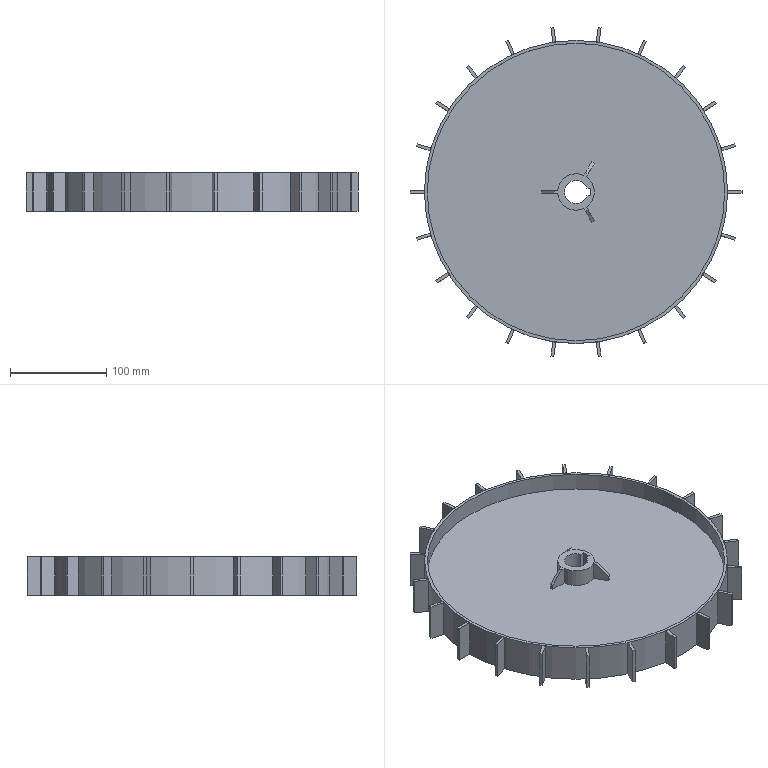Part | NX | features EXTRACT_BODY 21, EXTRUDE 5, CHAMFER 1, DATUM_CSYS 1, EXTRACT_DATUM_PLANE 1, Pattern Geometry 1, SKETCH 1, UNITE 1 | 24 solids | 175 faces | box 344.986 x 341.901 x 40 mm | volume 408899 mm3 | plane 143 | cylinder 32 | commonest cylinder face diameters 315 x23 38 x6 309 x2 24 x1